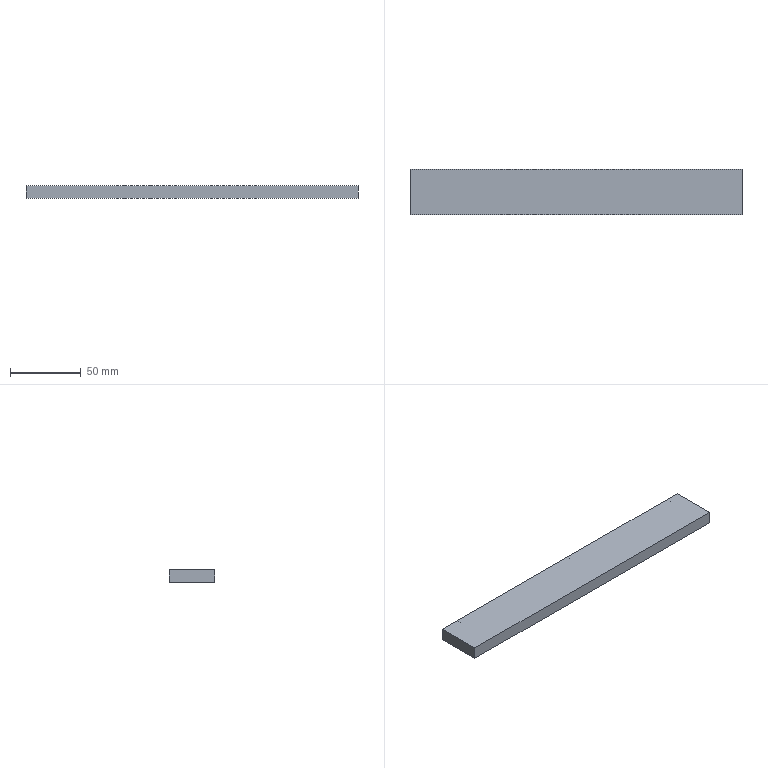Part | STEP file | BU-D02#180b | 1 solid | 37 faces | box 235 x 32.5 x 9 mm | volume 66956 mm3 | cylinder 19 | plane 12 | cone 6 | commonest cylinder face diameters 8 x7 3.3 x6 4.5 x6